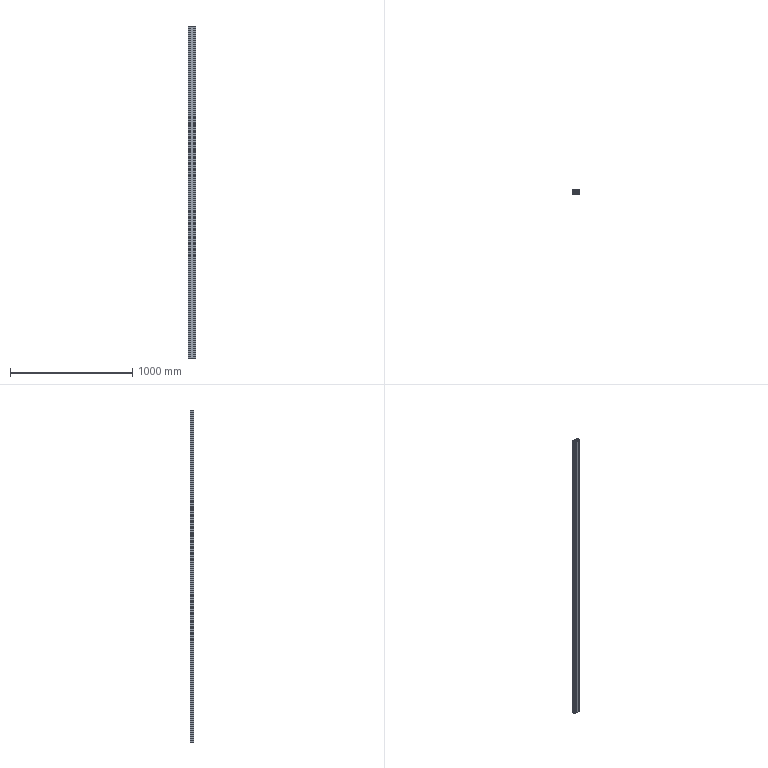Part | SolidWorks | features Cut 2, Extrusion 1 | 1 solid | 88 faces | box 60 x 30 x 2720 mm | volume 2264041 mm3 | plane 74 | cylinder 14 | commonest cylinder face diameters 24.431 x10 8.215 x4